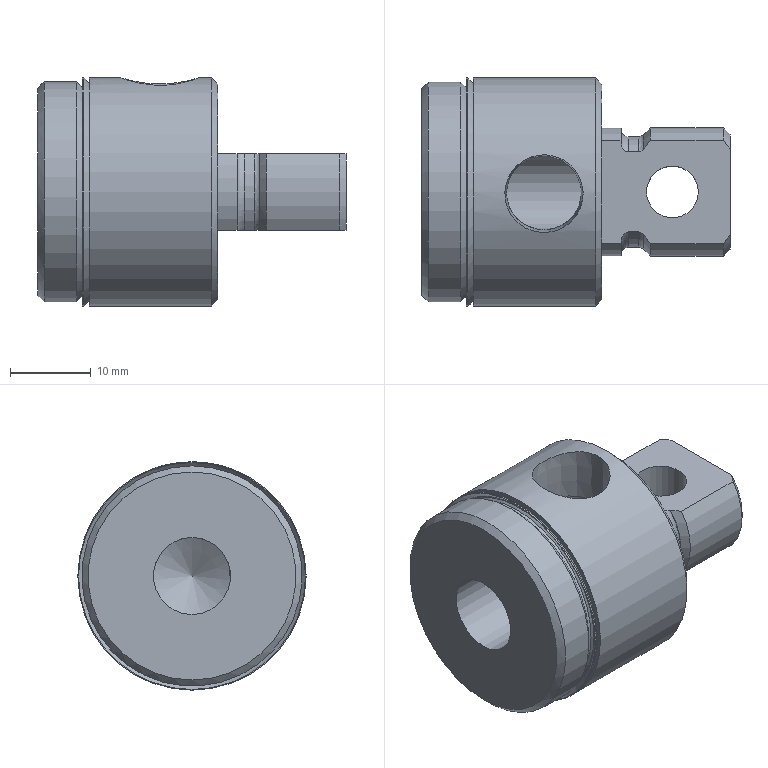Part | NX | features solid 2 | 1 solid | 41 faces | box 38.1 x 28.219 x 28.219 mm | volume 13145 mm3 | cone 14 | cylinder 13 | plane 9 | torus 5 | commonest cylinder face diameters 13.678 x2 15.812 x2 15.875 x2 28.219 x2 6.401 x1 9.246 x1
STEP:
#1=CARTESIAN_POINT('',(22.225,6.334,4.731));
#2=VERTEX_POINT('',#1);
#3=CARTESIAN_POINT('',(22.225,-6.334,4.731));
#4=VERTEX_POINT('',#3);
#5=CARTESIAN_POINT('',(22.225,28.219,4.731));
#6=DIRECTION('',(0.,-1.,0.));
#7=VECTOR('',#6,1000.);
#8=LINE('',#5,#7);
#9=EDGE_CURVE('',#2,#4,#8,.T.);
#10=ORIENTED_EDGE('',*,*,#9,.T.);
#11=CARTESIAN_POINT('',(24.613,-6.334,4.731));
#12=VERTEX_POINT('',#11);
#13=CARTESIAN_POINT('',(38.1,-6.334,4.731));
#14=DIRECTION('',(-1.,0.,0.));
#15=VECTOR('',#14,1000.);
#16=LINE('',#13,#15);
#17=EDGE_CURVE('',#12,#4,#16,.T.);
#18=ORIENTED_EDGE('',*,*,#17,.F.);
#19=CARTESIAN_POINT('',(24.613,-6.111,4.731));
#20=VERTEX_POINT('',#19);
#21=CARTESIAN_POINT('',(24.613,7.906,4.731));
#22=DIRECTION('',(0.,-1.,0.));
#23=VECTOR('',#22,1000.);
#24=LINE('',#21,#23);
#25=EDGE_CURVE('',#20,#12,#24,.T.);
#26=ORIENTED_EDGE('',*,*,#25,.F.);
#27=CARTESIAN_POINT('',(25.502,-4.939,4.731));
#28=VERTEX_POINT('',#27);
#29=CARTESIAN_POINT('',(24.613,-6.111,4.731));
#30=CARTESIAN_POINT('',(24.613,-5.842,4.731));
#31=CARTESIAN_POINT('',(24.751,-5.3,4.731));
#32=CARTESIAN_POINT('',(25.231,-4.939,4.731));
#33=CARTESIAN_POINT('',(25.502,-4.939,4.731));
#34=B_SPLINE_CURVE_WITH_KNOTS('',3,(#29,#30,#31,#32,#33),.UNSPECIFIED.,.F.,.F.,(4,1,4),(0.001401,0.002207,0.003014),.UNSPECIFIED.);
#35=EDGE_CURVE('',#20,#28,#34,.T.);
#36=ORIENTED_EDGE('',*,*,#35,.T.);
#37=CARTESIAN_POINT('',(26.784,-4.939,4.731));
#38=VERTEX_POINT('',#37);
#39=CARTESIAN_POINT('',(38.1,-4.939,4.731));
#40=DIRECTION('',(-1.,0.,0.));
#41=VECTOR('',#40,1000.);
#42=LINE('',#39,#41);
#43=EDGE_CURVE('',#38,#28,#42,.T.);
#44=ORIENTED_EDGE('',*,*,#43,.F.);
#45=CARTESIAN_POINT('',(27.383,-5.255,4.731));
#46=VERTEX_POINT('',#45);
#47=CARTESIAN_POINT('',(26.784,-4.939,4.731));
#48=CARTESIAN_POINT('',(27.017,-4.939,4.731));
#49=CARTESIAN_POINT('',(27.235,-5.073,4.731));
#50=CARTESIAN_POINT('',(27.383,-5.255,4.731));
#51=B_SPLINE_CURVE_WITH_KNOTS('',3,(#47,#48,#49,#50),.UNSPECIFIED.,.F.,.F.,(4,4),(0.003812,0.004508),.UNSPECIFIED.);
#52=EDGE_CURVE('',#38,#46,#51,.T.);
#53=ORIENTED_EDGE('',*,*,#52,.T.);
#54=CARTESIAN_POINT('',(27.413,-5.292,4.731));
#55=VERTEX_POINT('',#54);
#56=CARTESIAN_POINT('',(27.413,-5.292,4.731));
#57=CARTESIAN_POINT('',(27.403,-5.279,4.731));
#58=CARTESIAN_POINT('',(27.393,-5.267,4.731));
#59=CARTESIAN_POINT('',(27.383,-5.255,4.731));
#60=B_SPLINE_CURVE_WITH_KNOTS('',3,(#56,#57,#58,#59),.UNSPECIFIED.,.F.,.F.,(4,4),(0.01225,0.0123),.UNSPECIFIED.);
#61=EDGE_CURVE('',#55,#46,#60,.T.);
#62=ORIENTED_EDGE('',*,*,#61,.F.);
#63=CARTESIAN_POINT('',(28.252,-6.374,4.731));
#64=VERTEX_POINT('',#63);
#65=CARTESIAN_POINT('',(28.252,-6.374,4.731));
#66=CARTESIAN_POINT('',(27.967,-6.018,4.731));
#67=CARTESIAN_POINT('',(27.686,-5.658,4.731));
#68=CARTESIAN_POINT('',(27.413,-5.292,4.731));
#69=B_SPLINE_CURVE_WITH_KNOTS('',3,(#65,#66,#67,#68),.UNSPECIFIED.,.F.,.F.,(4,4),(0.01415,0.01552),.UNSPECIFIED.);
#70=EDGE_CURVE('',#64,#55,#69,.T.);
#71=ORIENTED_EDGE('',*,*,#70,.F.);
#72=CARTESIAN_POINT('',(37.261,-6.374,4.731));
#73=VERTEX_POINT('',#72);
#74=CARTESIAN_POINT('',(38.1,-6.374,4.731));
#75=DIRECTION('',(-1.,0.,0.));
#76=VECTOR('',#75,1000.);
#77=LINE('',#74,#76);
#78=EDGE_CURVE('',#73,#64,#77,.T.);
#79=ORIENTED_EDGE('',*,*,#78,.F.);
#80=CARTESIAN_POINT('',(38.1,-5.292,4.731));
#81=VERTEX_POINT('',#80);
#82=CARTESIAN_POINT('',(38.1,-5.292,4.731));
#83=CARTESIAN_POINT('',(37.828,-5.657,4.731));
#84=CARTESIAN_POINT('',(37.547,-6.017,4.731));
#85=CARTESIAN_POINT('',(37.261,-6.374,4.731));
#86=B_SPLINE_CURVE_WITH_KNOTS('',3,(#82,#83,#84,#85),.UNSPECIFIED.,.F.,.F.,(4,4),(0.02732,0.02869),.UNSPECIFIED.);
#87=EDGE_CURVE('',#81,#73,#86,.T.);
#88=ORIENTED_EDGE('',*,*,#87,.F.);
#89=CARTESIAN_POINT('',(38.1,5.292,4.731));
#90=VERTEX_POINT('',#89);
#91=CARTESIAN_POINT('',(38.1,28.219,4.731));
#92=DIRECTION('',(0.,-1.,0.));
#93=VECTOR('',#92,1000.);
#94=LINE('',#91,#93);
#95=EDGE_CURVE('',#90,#81,#94,.T.);
#96=ORIENTED_EDGE('',*,*,#95,.F.);
#97=CARTESIAN_POINT('',(37.261,6.374,4.731));
#98=VERTEX_POINT('',#97);
#99=CARTESIAN_POINT('',(37.261,6.374,4.731));
#100=CARTESIAN_POINT('',(37.546,6.018,4.731));
#101=CARTESIAN_POINT('',(37.827,5.658,4.731));
#102=CARTESIAN_POINT('',(38.1,5.292,4.731));
#103=B_SPLINE_CURVE_WITH_KNOTS('',3,(#99,#100,#101,#102),.UNSPECIFIED.,.F.,.F.,(4,4),(0.01415,0.01552),.UNSPECIFIED.);
#104=EDGE_CURVE('',#98,#90,#103,.T.);
#105=ORIENTED_EDGE('',*,*,#104,.F.);
#106=CARTESIAN_POINT('',(28.252,6.374,4.731));
#107=VERTEX_POINT('',#106);
#108=CARTESIAN_POINT('',(38.1,6.374,4.731));
#109=DIRECTION('',(-1.,0.,0.));
#110=VECTOR('',#109,1000.);
#111=LINE('',#108,#110);
#112=EDGE_CURVE('',#107,#98,#111,.F.);
#113=ORIENTED_EDGE('',*,*,#112,.F.);
#114=CARTESIAN_POINT('',(27.413,5.292,4.731));
#115=VERTEX_POINT('',#114);
#116=CARTESIAN_POINT('',(27.413,5.292,4.731));
#117=CARTESIAN_POINT('',(27.685,5.657,4.731));
#118=CARTESIAN_POINT('',(27.966,6.017,4.731));
#119=CARTESIAN_POINT('',(28.252,6.374,4.731));
#120=B_SPLINE_CURVE_WITH_KNOTS('',3,(#116,#117,#118,#119),.UNSPECIFIED.,.F.,.F.,(4,4),(0.02732,0.02869),.UNSPECIFIED.);
#121=EDGE_CURVE('',#115,#107,#120,.T.);
#122=ORIENTED_EDGE('',*,*,#121,.F.);
#123=CARTESIAN_POINT('',(27.383,5.255,4.731));
#124=VERTEX_POINT('',#123);
#125=CARTESIAN_POINT('',(27.383,5.255,4.731));
#126=CARTESIAN_POINT('',(27.393,5.267,4.731));
#127=CARTESIAN_POINT('',(27.403,5.279,4.731));
#128=CARTESIAN_POINT('',(27.413,5.292,4.731));
#129=B_SPLINE_CURVE_WITH_KNOTS('',3,(#125,#126,#127,#128),.UNSPECIFIED.,.F.,.F.,(4,4),(0.02417,0.02422),.UNSPECIFIED.);
#130=EDGE_CURVE('',#124,#115,#129,.T.);
#131=ORIENTED_EDGE('',*,*,#130,.F.);
#132=CARTESIAN_POINT('',(26.784,4.939,4.731));
#133=VERTEX_POINT('',#132);
#134=CARTESIAN_POINT('',(27.383,5.255,4.731));
#135=CARTESIAN_POINT('',(27.236,5.075,4.731));
#136=CARTESIAN_POINT('',(27.018,4.939,4.731));
#137=CARTESIAN_POINT('',(26.784,4.939,4.731));
#138=B_SPLINE_CURVE_WITH_KNOTS('',3,(#134,#135,#136,#137),.UNSPECIFIED.,.F.,.F.,(4,4),(0.005905,0.0066),.UNSPECIFIED.);
#139=EDGE_CURVE('',#124,#133,#138,.T.);
#140=ORIENTED_EDGE('',*,*,#139,.T.);
#141=CARTESIAN_POINT('',(25.502,4.939,4.731));
#142=VERTEX_POINT('',#141);
#143=CARTESIAN_POINT('',(38.1,4.939,4.731));
#144=DIRECTION('',(-1.,0.,0.));
#145=VECTOR('',#144,1000.);
#146=LINE('',#143,#145);
#147=EDGE_CURVE('',#142,#133,#146,.F.);
#148=ORIENTED_EDGE('',*,*,#147,.F.);
#149=CARTESIAN_POINT('',(24.613,6.111,4.731));
#150=VERTEX_POINT('',#149);
#151=CARTESIAN_POINT('',(25.502,4.939,4.731));
#152=CARTESIAN_POINT('',(25.232,4.939,4.731));
#153=CARTESIAN_POINT('',(24.751,5.299,4.731));
#154=CARTESIAN_POINT('',(24.613,5.842,4.731));
#155=CARTESIAN_POINT('',(24.613,6.111,4.731));
#156=B_SPLINE_CURVE_WITH_KNOTS('',3,(#151,#152,#153,#154,#155),.UNSPECIFIED.,.F.,.F.,(4,1,4),(0.006205,0.007011,0.007818),.UNSPECIFIED.);
#157=EDGE_CURVE('',#142,#150,#156,.T.);
#158=ORIENTED_EDGE('',*,*,#157,.T.);
#159=CARTESIAN_POINT('',(24.613,6.334,4.731));
#160=VERTEX_POINT('',#159);
#161=CARTESIAN_POINT('',(24.613,7.906,4.731));
#162=DIRECTION('',(0.,-1.,0.));
#163=VECTOR('',#162,1000.);
#164=LINE('',#161,#163);
#165=EDGE_CURVE('',#160,#150,#164,.T.);
#166=ORIENTED_EDGE('',*,*,#165,.F.);
#167=CARTESIAN_POINT('',(38.1,6.334,4.731));
#168=DIRECTION('',(-1.,0.,0.));
#169=VECTOR('',#168,1000.);
#170=LINE('',#167,#169);
#171=EDGE_CURVE('',#2,#160,#170,.F.);
#172=ORIENTED_EDGE('',*,*,#171,.F.);
#173=EDGE_LOOP('',(#10,#18,#26,#36,#44,#53,#62,#71,#79,#88,#96,#105,#113,#122,#131,#140,#148,#158,#166,#172));
#174=FACE_BOUND('',#173,.T.);
#175=CARTESIAN_POINT('',(34.163,0.,4.731));
#176=VERTEX_POINT('',#175);
#177=CARTESIAN_POINT('',(30.963,0.,4.731));
#178=DIRECTION('',(0.,0.,1.));
#179=DIRECTION('',(1.,0.,0.));
#180=AXIS2_PLACEMENT_3D('',#177,#178,#179);
#181=CIRCLE('',#180,3.2);
#182=EDGE_CURVE('',#176,#176,#181,.F.);
#183=ORIENTED_EDGE('',*,*,#182,.T.);
#184=EDGE_LOOP('',(#183));
#185=FACE_BOUND('',#184,.T.);
#186=CARTESIAN_POINT('',(22.225,28.219,4.731));
#187=DIRECTION('',(0.,0.,1.));
#188=DIRECTION('',(1.,0.,0.));
#189=AXIS2_PLACEMENT_3D('',#186,#187,#188);
#190=PLANE('',#189);
#191=ADVANCED_FACE('',(#174,#185),#190,.T.);
#192=CARTESIAN_POINT('',(22.225,-6.334,-4.731));
#193=VERTEX_POINT('',#192);
#194=CARTESIAN_POINT('',(22.225,6.334,-4.731));
#195=VERTEX_POINT('',#194);
#196=CARTESIAN_POINT('',(22.225,-28.219,-4.731));
#197=DIRECTION('',(0.,1.,0.));
#198=VECTOR('',#197,1000.);
#199=LINE('',#196,#198);
#200=EDGE_CURVE('',#193,#195,#199,.T.);
#201=ORIENTED_EDGE('',*,*,#200,.T.);
#202=CARTESIAN_POINT('',(24.613,6.334,-4.731));
#203=VERTEX_POINT('',#202);
#204=CARTESIAN_POINT('',(38.1,6.334,-4.731));
#205=DIRECTION('',(-1.,0.,0.));
#206=VECTOR('',#205,1000.);
#207=LINE('',#204,#206);
#208=EDGE_CURVE('',#203,#195,#207,.T.);
#209=ORIENTED_EDGE('',*,*,#208,.F.);
#210=CARTESIAN_POINT('',(24.613,6.111,-4.731));
#211=VERTEX_POINT('',#210);
#212=CARTESIAN_POINT('',(24.613,7.906,-4.731));
#213=DIRECTION('',(0.,1.,0.));
#214=VECTOR('',#213,1000.);
#215=LINE('',#212,#214);
#216=EDGE_CURVE('',#211,#203,#215,.T.);
#217=ORIENTED_EDGE('',*,*,#216,.F.);
#218=CARTESIAN_POINT('',(25.502,4.939,-4.731));
#219=VERTEX_POINT('',#218);
#220=CARTESIAN_POINT('',(24.613,6.111,-4.731));
#221=CARTESIAN_POINT('',(24.613,5.839,-4.731));
#222=CARTESIAN_POINT('',(24.75,5.302,-4.731));
#223=CARTESIAN_POINT('',(25.232,4.939,-4.731));
#224=CARTESIAN_POINT('',(25.502,4.939,-4.731));
#225=B_SPLINE_CURVE_WITH_KNOTS('',3,(#220,#221,#222,#223,#224),.UNSPECIFIED.,.F.,.F.,(4,1,4),(0.004854,0.005662,0.006469),.UNSPECIFIED.);
#226=EDGE_CURVE('',#211,#219,#225,.T.);
#227=ORIENTED_EDGE('',*,*,#226,.T.);
#228=CARTESIAN_POINT('',(26.784,4.939,-4.731));
#229=VERTEX_POINT('',#228);
#230=CARTESIAN_POINT('',(38.1,4.939,-4.731));
#231=DIRECTION('',(-1.,0.,0.));
#232=VECTOR('',#231,1000.);
#233=LINE('',#230,#232);
#234=EDGE_CURVE('',#229,#219,#233,.T.);
#235=ORIENTED_EDGE('',*,*,#234,.F.);
#236=CARTESIAN_POINT('',(27.383,5.255,-4.731));
#237=VERTEX_POINT('',#236);
#238=CARTESIAN_POINT('',(26.784,4.939,-4.731));
#239=CARTESIAN_POINT('',(27.017,4.939,-4.731));
#240=CARTESIAN_POINT('',(27.237,5.076,-4.731));
#241=CARTESIAN_POINT('',(27.383,5.255,-4.731));
#242=B_SPLINE_CURVE_WITH_KNOTS('',3,(#238,#239,#240,#241),.UNSPECIFIED.,.F.,.F.,(4,4),(0.00608,0.006774),.UNSPECIFIED.);
#243=EDGE_CURVE('',#229,#237,#242,.T.);
#244=ORIENTED_EDGE('',*,*,#243,.T.);
#245=CARTESIAN_POINT('',(27.413,5.292,-4.731));
#246=VERTEX_POINT('',#245);
#247=CARTESIAN_POINT('',(27.413,5.292,-4.731));
#248=CARTESIAN_POINT('',(27.403,5.279,-4.731));
#249=CARTESIAN_POINT('',(27.393,5.267,-4.731));
#250=CARTESIAN_POINT('',(27.383,5.255,-4.731));
#251=B_SPLINE_CURVE_WITH_KNOTS('',3,(#247,#248,#249,#250),.UNSPECIFIED.,.F.,.F.,(4,4),(0.01225,0.0123),.UNSPECIFIED.);
#252=EDGE_CURVE('',#246,#237,#251,.T.);
#253=ORIENTED_EDGE('',*,*,#252,.F.);
#254=CARTESIAN_POINT('',(28.252,6.374,-4.731));
#255=VERTEX_POINT('',#254);
#256=CARTESIAN_POINT('',(28.252,6.374,-4.731));
#257=CARTESIAN_POINT('',(27.967,6.018,-4.731));
#258=CARTESIAN_POINT('',(27.686,5.658,-4.731));
#259=CARTESIAN_POINT('',(27.413,5.292,-4.731));
#260=B_SPLINE_CURVE_WITH_KNOTS('',3,(#256,#257,#258,#259),.UNSPECIFIED.,.F.,.F.,(4,4),(0.01415,0.01552),.UNSPECIFIED.);
#261=EDGE_CURVE('',#255,#246,#260,.T.);
#262=ORIENTED_EDGE('',*,*,#261,.F.);
#263=CARTESIAN_POINT('',(37.261,6.374,-4.731));
#264=VERTEX_POINT('',#263);
#265=CARTESIAN_POINT('',(38.1,6.374,-4.731));
#266=DIRECTION('',(-1.,0.,0.));
#267=VECTOR('',#266,1000.);
#268=LINE('',#265,#267);
#269=EDGE_CURVE('',#264,#255,#268,.T.);
#270=ORIENTED_EDGE('',*,*,#269,.F.);
#271=CARTESIAN_POINT('',(38.1,5.292,-4.731));
#272=VERTEX_POINT('',#271);
#273=CARTESIAN_POINT('',(38.1,5.292,-4.731));
#274=CARTESIAN_POINT('',(37.828,5.657,-4.731));
#275=CARTESIAN_POINT('',(37.547,6.017,-4.731));
#276=CARTESIAN_POINT('',(37.261,6.374,-4.731));
#277=B_SPLINE_CURVE_WITH_KNOTS('',3,(#273,#274,#275,#276),.UNSPECIFIED.,.F.,.F.,(4,4),(0.02732,0.02869),.UNSPECIFIED.);
#278=EDGE_CURVE('',#272,#264,#277,.T.);
#279=ORIENTED_EDGE('',*,*,#278,.F.);
#280=CARTESIAN_POINT('',(38.1,-5.292,-4.731));
#281=VERTEX_POINT('',#280);
#282=CARTESIAN_POINT('',(38.1,-28.219,-4.731));
#283=DIRECTION('',(0.,1.,0.));
#284=VECTOR('',#283,1000.);
#285=LINE('',#282,#284);
#286=EDGE_CURVE('',#281,#272,#285,.T.);
#287=ORIENTED_EDGE('',*,*,#286,.F.);
#288=CARTESIAN_POINT('',(37.261,-6.374,-4.731));
#289=VERTEX_POINT('',#288);
#290=CARTESIAN_POINT('',(37.261,-6.374,-4.731));
#291=CARTESIAN_POINT('',(37.546,-6.018,-4.731));
#292=CARTESIAN_POINT('',(37.827,-5.658,-4.731));
#293=CARTESIAN_POINT('',(38.1,-5.292,-4.731));
#294=B_SPLINE_CURVE_WITH_KNOTS('',3,(#290,#291,#292,#293),.UNSPECIFIED.,.F.,.F.,(4,4),(0.01415,0.01552),.UNSPECIFIED.);
#295=EDGE_CURVE('',#289,#281,#294,.T.);
#296=ORIENTED_EDGE('',*,*,#295,.F.);
#297=CARTESIAN_POINT('',(28.252,-6.374,-4.731));
#298=VERTEX_POINT('',#297);
#299=CARTESIAN_POINT('',(38.1,-6.374,-4.731));
#300=DIRECTION('',(-1.,0.,0.));
#301=VECTOR('',#300,1000.);
#302=LINE('',#299,#301);
#303=EDGE_CURVE('',#298,#289,#302,.F.);
#304=ORIENTED_EDGE('',*,*,#303,.F.);
#305=CARTESIAN_POINT('',(27.413,-5.292,-4.731));
#306=VERTEX_POINT('',#305);
#307=CARTESIAN_POINT('',(27.413,-5.292,-4.731));
#308=CARTESIAN_POINT('',(27.685,-5.657,-4.731));
#309=CARTESIAN_POINT('',(27.966,-6.017,-4.731));
#310=CARTESIAN_POINT('',(28.252,-6.374,-4.731));
#311=B_SPLINE_CURVE_WITH_KNOTS('',3,(#307,#308,#309,#310),.UNSPECIFIED.,.F.,.F.,(4,4),(0.02732,0.02869),.UNSPECIFIED.);
#312=EDGE_CURVE('',#306,#298,#311,.T.);
#313=ORIENTED_EDGE('',*,*,#312,.F.);
#314=CARTESIAN_POINT('',(27.383,-5.255,-4.731));
#315=VERTEX_POINT('',#314);
#316=CARTESIAN_POINT('',(27.383,-5.255,-4.731));
#317=CARTESIAN_POINT('',(27.393,-5.267,-4.731));
#318=CARTESIAN_POINT('',(27.403,-5.279,-4.731));
#319=CARTESIAN_POINT('',(27.413,-5.292,-4.731));
#320=B_SPLINE_CURVE_WITH_KNOTS('',3,(#316,#317,#318,#319),.UNSPECIFIED.,.F.,.F.,(4,4),(0.02417,0.02422),.UNSPECIFIED.);
#321=EDGE_CURVE('',#315,#306,#320,.T.);
#322=ORIENTED_EDGE('',*,*,#321,.F.);
#323=CARTESIAN_POINT('',(26.784,-4.939,-4.731));
#324=VERTEX_POINT('',#323);
#325=CARTESIAN_POINT('',(27.383,-5.255,-4.731));
#326=CARTESIAN_POINT('',(27.236,-5.075,-4.731));
#327=CARTESIAN_POINT('',(27.017,-4.939,-4.731));
#328=CARTESIAN_POINT('',(26.784,-4.939,-4.731));
#329=B_SPLINE_CURVE_WITH_KNOTS('',3,(#325,#326,#327,#328),.UNSPECIFIED.,.F.,.F.,(4,4),(0.00183,0.002524),.UNSPECIFIED.);
#330=EDGE_CURVE('',#315,#324,#329,.T.);
#331=ORIENTED_EDGE('',*,*,#330,.T.);
#332=CARTESIAN_POINT('',(25.502,-4.939,-4.731));
#333=VERTEX_POINT('',#332);
#334=CARTESIAN_POINT('',(38.1,-4.939,-4.731));
#335=DIRECTION('',(-1.,0.,0.));
#336=VECTOR('',#335,1000.);
#337=LINE('',#334,#336);
#338=EDGE_CURVE('',#333,#324,#337,.F.);
#339=ORIENTED_EDGE('',*,*,#338,.F.);
#340=CARTESIAN_POINT('',(24.613,-6.111,-4.731));
#341=VERTEX_POINT('',#340);
#342=CARTESIAN_POINT('',(25.502,-4.939,-4.731));
#343=CARTESIAN_POINT('',(25.233,-4.939,-4.731));
#344=CARTESIAN_POINT('',(24.751,-5.299,-4.731));
#345=CARTESIAN_POINT('',(24.613,-5.843,-4.731));
#346=CARTESIAN_POINT('',(24.613,-6.111,-4.731));
#347=B_SPLINE_CURVE_WITH_KNOTS('',3,(#342,#343,#344,#345,#346),.UNSPECIFIED.,.F.,.F.,(4,1,4),(0.003324,0.004131,0.004938),.UNSPECIFIED.);
#348=EDGE_CURVE('',#333,#341,#347,.T.);
#349=ORIENTED_EDGE('',*,*,#348,.T.);
#350=CARTESIAN_POINT('',(24.613,-6.334,-4.731));
#351=VERTEX_POINT('',#350);
#352=CARTESIAN_POINT('',(24.613,7.906,-4.731));
#353=DIRECTION('',(0.,1.,0.));
#354=VECTOR('',#353,1000.);
#355=LINE('',#352,#354);
#356=EDGE_CURVE('',#351,#341,#355,.T.);
#357=ORIENTED_EDGE('',*,*,#356,.F.);
#358=CARTESIAN_POINT('',(38.1,-6.334,-4.731));
#359=DIRECTION('',(-1.,0.,0.));
#360=VECTOR('',#359,1000.);
#361=LINE('',#358,#360);
#362=EDGE_CURVE('',#193,#351,#361,.F.);
#363=ORIENTED_EDGE('',*,*,#362,.F.);
#364=EDGE_LOOP('',(#201,#209,#217,#227,#235,#244,#253,#262,#270,#279,#287,#296,#304,#313,#322,#331,#339,#349,#357,#363));
#365=FACE_BOUND('',#364,.T.);
#366=CARTESIAN_POINT('',(27.762,0.,-4.731));
#367=VERTEX_POINT('',#366);
#368=CARTESIAN_POINT('',(30.963,0.,-4.731));
#369=DIRECTION('',(0.,0.,-1.));
#370=DIRECTION('',(-1.,0.,0.));
#371=AXIS2_PLACEMENT_3D('',#368,#369,#370);
#372=CIRCLE('',#371,3.2);
#373=EDGE_CURVE('',#367,#367,#372,.F.);
#374=ORIENTED_EDGE('',*,*,#373,.T.);
#375=EDGE_LOOP('',(#374));
#376=FACE_BOUND('',#375,.T.);
#377=CARTESIAN_POINT('',(22.225,-28.219,-4.731));
#378=DIRECTION('',(0.,0.,-1.));
#379=DIRECTION('',(-1.,0.,0.));
#380=AXIS2_PLACEMENT_3D('',#377,#378,#379);
#381=PLANE('',#380);
#382=ADVANCED_FACE('',(#365,#376),#381,.T.);
#383=CARTESIAN_POINT('',(5.588,0.,12.846));
#384=VERTEX_POINT('',#383);
#385=CARTESIAN_POINT('',(5.588,0.,0.));
#386=DIRECTION('',(-1.,0.,0.));
#387=DIRECTION('',(0.,0.,1.));
#388=AXIS2_PLACEMENT_3D('',#385,#386,#387);
#389=CIRCLE('',#388,12.846);
#390=EDGE_CURVE('',#384,#384,#389,.T.);
#391=ORIENTED_EDGE('',*,*,#390,.F.);
#392=EDGE_LOOP('',(#391));
#393=FACE_BOUND('',#392,.T.);
#394=CARTESIAN_POINT('',(5.969,-12.846,0.));
#395=VERTEX_POINT('',#394);
#396=CARTESIAN_POINT('',(5.969,0.,0.));
#397=DIRECTION('',(-1.,0.,0.));
#398=DIRECTION('',(0.,-1.,0.));
#399=AXIS2_PLACEMENT_3D('',#396,#397,#398);
#400=CIRCLE('',#399,12.846);
#401=EDGE_CURVE('',#395,#395,#400,.T.);
#402=ORIENTED_EDGE('',*,*,#401,.T.);
#403=EDGE_LOOP('',(#402));
#404=FACE_BOUND('',#403,.T.);
#405=CARTESIAN_POINT('',(22.225,0.,0.));
#406=DIRECTION('',(-1.,0.,0.));
#407=DIRECTION('',(0.,0.,1.));
#408=AXIS2_PLACEMENT_3D('',#405,#406,#407);
#409=CYLINDRICAL_SURFACE('',#408,12.846);
#410=ADVANCED_FACE('',(#393,#404),#409,.T.);
#411=CARTESIAN_POINT('',(6.35,0.,14.11));
#412=VERTEX_POINT('',#411);
#413=CARTESIAN_POINT('',(6.35,0.,0.));
#414=DIRECTION('',(-1.,0.,0.));
#415=DIRECTION('',(0.,0.,1.));
#416=AXIS2_PLACEMENT_3D('',#413,#414,#415);
#417=CIRCLE('',#416,14.11);
#418=EDGE_CURVE('',#412,#412,#417,.T.);
#419=ORIENTED_EDGE('',*,*,#418,.T.);
#420=EDGE_LOOP('',(#419));
#421=FACE_BOUND('',#420,.T.);
#422=CARTESIAN_POINT('',(6.35,-13.449,0.));
#423=VERTEX_POINT('',#422);
#424=CARTESIAN_POINT('',(6.35,0.,0.));
#425=DIRECTION('',(-1.,0.,0.));
#426=DIRECTION('',(0.,-1.,0.));
#427=AXIS2_PLACEMENT_3D('',#424,#425,#426);
#428=CIRCLE('',#427,13.449);
#429=EDGE_CURVE('',#423,#423,#428,.T.);
#430=ORIENTED_EDGE('',*,*,#429,.F.);
#431=EDGE_LOOP('',(#430));
#432=FACE_BOUND('',#431,.T.);
#433=CARTESIAN_POINT('',(6.35,12.846,0.));
#434=DIRECTION('',(-1.,0.,0.));
#435=DIRECTION('',(0.,0.,1.));
#436=AXIS2_PLACEMENT_3D('',#433,#434,#435);
#437=PLANE('',#436);
#438=ADVANCED_FACE('',(#421,#432),#437,.T.);
#439=CARTESIAN_POINT('',(22.225,0.,0.));
#440=DIRECTION('',(1.,0.,0.));
#441=DIRECTION('',(0.,0.,-1.));
#442=AXIS2_PLACEMENT_3D('',#439,#440,#441);
#443=CIRCLE('',#442,7.906);
#444=EDGE_CURVE('',#4,#193,#443,.T.);
#445=ORIENTED_EDGE('',*,*,#444,.T.);
#446=ORIENTED_EDGE('',*,*,#362,.T.);
#447=CARTESIAN_POINT('',(24.613,0.,0.));
#448=DIRECTION('',(-1.,0.,0.));
#449=DIRECTION('',(0.,0.,1.));
#450=AXIS2_PLACEMENT_3D('',#447,#448,#449);
#451=CIRCLE('',#450,7.906);
#452=EDGE_CURVE('',#351,#12,#451,.T.);
#453=ORIENTED_EDGE('',*,*,#452,.T.);
#454=ORIENTED_EDGE('',*,*,#17,.T.);
#455=EDGE_LOOP('',(#445,#446,#453,#454));
#456=FACE_BOUND('',#455,.T.);
#457=CARTESIAN_POINT('',(38.1,0.,0.));
#458=DIRECTION('',(-1.,0.,0.));
#459=DIRECTION('',(0.,0.,1.));
#460=AXIS2_PLACEMENT_3D('',#457,#458,#459);
#461=CYLINDRICAL_SURFACE('',#460,7.906);
#462=ADVANCED_FACE('',(#456),#461,.T.);
#463=CARTESIAN_POINT('',(24.613,0.,0.));
#464=DIRECTION('',(-1.,0.,0.));
#465=DIRECTION('',(0.,0.,1.));
#466=AXIS2_PLACEMENT_3D('',#463,#464,#465);
#467=CIRCLE('',#466,7.906);
#468=EDGE_CURVE('',#160,#203,#467,.T.);
#469=ORIENTED_EDGE('',*,*,#468,.T.);
#470=ORIENTED_EDGE('',*,*,#208,.T.);
#471=CARTESIAN_POINT('',(22.225,0.,0.));
#472=DIRECTION('',(1.,0.,0.));
#473=DIRECTION('',(0.,0.,-1.));
#474=AXIS2_PLACEMENT_3D('',#471,#472,#473);
#475=CIRCLE('',#474,7.906);
#476=EDGE_CURVE('',#195,#2,#475,.T.);
#477=ORIENTED_EDGE('',*,*,#476,.T.);
#478=ORIENTED_EDGE('',*,*,#171,.T.);
#479=EDGE_LOOP('',(#469,#470,#477,#478));
#480=FACE_BOUND('',#479,.T.);
#481=CARTESIAN_POINT('',(38.1,0.,0.));
#482=DIRECTION('',(-1.,0.,0.));
#483=DIRECTION('',(0.,0.,1.));
#484=AXIS2_PLACEMENT_3D('',#481,#482,#483);
#485=CYLINDRICAL_SURFACE('',#484,7.906);
#486=ADVANCED_FACE('',(#480),#485,.T.);
#487=ORIENTED_EDGE('',*,*,#452,.F.);
#488=ORIENTED_EDGE('',*,*,#356,.T.);
#489=CARTESIAN_POINT('',(24.613,0.,0.));
#490=DIRECTION('',(-1.,0.,0.));
#491=DIRECTION('',(0.,0.,1.));
#492=AXIS2_PLACEMENT_3D('',#489,#490,#491);
#493=CIRCLE('',#492,7.728);
#494=EDGE_CURVE('',#341,#20,#493,.T.);
#495=ORIENTED_EDGE('',*,*,#494,.T.);
#496=ORIENTED_EDGE('',*,*,#25,.T.);
#497=EDGE_LOOP('',(#487,#488,#495,#496));
#498=FACE_BOUND('',#497,.T.);
#499=CARTESIAN_POINT('',(24.613,7.906,0.));
#500=DIRECTION('',(1.,0.,0.));
#501=DIRECTION('',(0.,0.,-1.));
#502=AXIS2_PLACEMENT_3D('',#499,#500,#501);
#503=PLANE('',#502);
#504=ADVANCED_FACE('',(#498),#503,.T.);
#505=CARTESIAN_POINT('',(24.613,0.,0.));
#506=DIRECTION('',(-1.,0.,0.));
#507=DIRECTION('',(0.,0.,1.));
#508=AXIS2_PLACEMENT_3D('',#505,#506,#507);
#509=CIRCLE('',#508,7.728);
#510=EDGE_CURVE('',#150,#211,#509,.T.);
#511=ORIENTED_EDGE('',*,*,#510,.T.);
#512=ORIENTED_EDGE('',*,*,#216,.T.);
#513=ORIENTED_EDGE('',*,*,#468,.F.);
#514=ORIENTED_EDGE('',*,*,#165,.T.);
#515=EDGE_LOOP('',(#511,#512,#513,#514));
#516=FACE_BOUND('',#515,.T.);
#517=CARTESIAN_POINT('',(24.613,7.906,0.));
#518=DIRECTION('',(1.,0.,0.));
#519=DIRECTION('',(0.,0.,-1.));
#520=AXIS2_PLACEMENT_3D('',#517,#518,#519);
#521=PLANE('',#520);
#522=ADVANCED_FACE('',(#516),#521,.T.);
#523=ORIENTED_EDGE('',*,*,#348,.F.);
#524=CARTESIAN_POINT('',(25.502,0.,0.));
#525=DIRECTION('',(-1.,0.,0.));
#526=DIRECTION('',(0.,0.,1.));
#527=AXIS2_PLACEMENT_3D('',#524,#525,#526);
#528=CIRCLE('',#527,6.839);
#529=EDGE_CURVE('',#333,#28,#528,.T.);
#530=ORIENTED_EDGE('',*,*,#529,.T.);
#531=ORIENTED_EDGE('',*,*,#35,.F.);
#532=ORIENTED_EDGE('',*,*,#494,.F.);
#533=EDGE_LOOP('',(#523,#530,#531,#532));
#534=FACE_BOUND('',#533,.T.);
#535=CARTESIAN_POINT('',(25.502,0.,0.));
#536=DIRECTION('',(-1.,0.,0.));
#537=DIRECTION('',(0.,0.,1.));
#538=AXIS2_PLACEMENT_3D('',#535,#536,#537);
#539=TOROIDAL_SURFACE('',#538,7.728,0.889);
#540=ADVANCED_FACE('',(#534),#539,.F.);
#541=ORIENTED_EDGE('',*,*,#226,.F.);
#542=ORIENTED_EDGE('',*,*,#510,.F.);
#543=ORIENTED_EDGE('',*,*,#157,.F.);
#544=CARTESIAN_POINT('',(25.502,0.,0.));
#545=DIRECTION('',(-1.,0.,0.));
#546=DIRECTION('',(0.,0.,1.));
#547=AXIS2_PLACEMENT_3D('',#544,#545,#546);
#548=CIRCLE('',#547,6.839);
#549=EDGE_CURVE('',#142,#219,#548,.T.);
#550=ORIENTED_EDGE('',*,*,#549,.T.);
#551=EDGE_LOOP('',(#541,#542,#543,#550));
#552=FACE_BOUND('',#551,.T.);
#553=CARTESIAN_POINT('',(25.502,0.,0.));
#554=DIRECTION('',(-1.,0.,0.));
#555=DIRECTION('',(0.,0.,1.));
#556=AXIS2_PLACEMENT_3D('',#553,#554,#555);
#557=TOROIDAL_SURFACE('',#556,7.728,0.889);
#558=ADVANCED_FACE('',(#552),#557,.F.);
#559=ORIENTED_EDGE('',*,*,#529,.F.);
#560=ORIENTED_EDGE('',*,*,#338,.T.);
#561=CARTESIAN_POINT('',(26.784,0.,0.));
#562=DIRECTION('',(-1.,0.,0.));
#563=DIRECTION('',(0.,0.,1.));
#564=AXIS2_PLACEMENT_3D('',#561,#562,#563);
#565=CIRCLE('',#564,6.839);
#566=EDGE_CURVE('',#324,#38,#565,.T.);
#567=ORIENTED_EDGE('',*,*,#566,.T.);
#568=ORIENTED_EDGE('',*,*,#43,.T.);
#569=EDGE_LOOP('',(#559,#560,#567,#568));
#570=FACE_BOUND('',#569,.T.);
#571=CARTESIAN_POINT('',(38.1,0.,0.));
#572=DIRECTION('',(-1.,0.,0.));
#573=DIRECTION('',(0.,0.,1.));
#574=AXIS2_PLACEMENT_3D('',#571,#572,#573);
#575=CYLINDRICAL_SURFACE('',#574,6.839);
#576=ADVANCED_FACE('',(#570),#575,.T.);
#577=CARTESIAN_POINT('',(26.784,0.,0.));
#578=DIRECTION('',(-1.,0.,0.));
#579=DIRECTION('',(0.,0.,1.));
#580=AXIS2_PLACEMENT_3D('',#577,#578,#579);
#581=CIRCLE('',#580,6.839);
#582=EDGE_CURVE('',#133,#229,#581,.T.);
#583=ORIENTED_EDGE('',*,*,#582,.T.);
#584=ORIENTED_EDGE('',*,*,#234,.T.);
#585=ORIENTED_EDGE('',*,*,#549,.F.);
#586=ORIENTED_EDGE('',*,*,#147,.T.);
#587=EDGE_LOOP('',(#583,#584,#585,#586));
#588=FACE_BOUND('',#587,.T.);
#589=CARTESIAN_POINT('',(38.1,0.,0.));
#590=DIRECTION('',(-1.,0.,0.));
#591=DIRECTION('',(0.,0.,1.));
#592=AXIS2_PLACEMENT_3D('',#589,#590,#591);
#593=CYLINDRICAL_SURFACE('',#592,6.839);
#594=ADVANCED_FACE('',(#588),#593,.T.);
#595=ORIENTED_EDGE('',*,*,#330,.F.);
#596=CARTESIAN_POINT('',(27.383,0.,0.));
#597=DIRECTION('',(-1.,0.,0.));
#598=DIRECTION('',(0.,0.,1.));
#599=AXIS2_PLACEMENT_3D('',#596,#597,#598);
#600=CIRCLE('',#599,7.071);
#601=EDGE_CURVE('',#315,#46,#600,.T.);
#602=ORIENTED_EDGE('',*,*,#601,.T.);
#603=ORIENTED_EDGE('',*,*,#52,.F.);
#604=ORIENTED_EDGE('',*,*,#566,.F.);
#605=EDGE_LOOP('',(#595,#602,#603,#604));
#606=FACE_BOUND('',#605,.T.);
#607=CARTESIAN_POINT('',(26.784,0.,0.));
#608=DIRECTION('',(-1.,0.,0.));
#609=DIRECTION('',(0.,0.,1.));
#610=AXIS2_PLACEMENT_3D('',#607,#608,#609);
#611=TOROIDAL_SURFACE('',#610,7.728,0.889);
#612=ADVANCED_FACE('',(#606),#611,.F.);
#613=ORIENTED_EDGE('',*,*,#243,.F.);
#614=ORIENTED_EDGE('',*,*,#582,.F.);
#615=ORIENTED_EDGE('',*,*,#139,.F.);
#616=CARTESIAN_POINT('',(27.383,0.,0.));
#617=DIRECTION('',(-1.,0.,0.));
#618=DIRECTION('',(0.,0.,1.));
#619=AXIS2_PLACEMENT_3D('',#616,#617,#618);
#620=CIRCLE('',#619,7.071);
#621=EDGE_CURVE('',#124,#237,#620,.T.);
#622=ORIENTED_EDGE('',*,*,#621,.T.);
#623=EDGE_LOOP('',(#613,#614,#615,#622));
#624=FACE_BOUND('',#623,.T.);
#625=CARTESIAN_POINT('',(26.784,0.,0.));
#626=DIRECTION('',(-1.,0.,0.));
#627=DIRECTION('',(0.,0.,1.));
#628=AXIS2_PLACEMENT_3D('',#625,#626,#627);
#629=TOROIDAL_SURFACE('',#628,7.728,0.889);
#630=ADVANCED_FACE('',(#624),#629,.F.);
#631=CARTESIAN_POINT('',(27.413,0.,0.));
#632=DIRECTION('',(-1.,0.,0.));
#633=DIRECTION('',(0.,0.,1.));
#634=AXIS2_PLACEMENT_3D('',#631,#632,#633);
#635=CIRCLE('',#634,7.098);
#636=EDGE_CURVE('',#115,#246,#635,.T.);
#637=ORIENTED_EDGE('',*,*,#636,.T.);
#638=ORIENTED_EDGE('',*,*,#252,.T.);
#639=ORIENTED_EDGE('',*,*,#621,.F.);
#640=ORIENTED_EDGE('',*,*,#130,.T.);
#641=EDGE_LOOP('',(#637,#638,#639,#640));
#642=FACE_BOUND('',#641,.T.);
#643=CARTESIAN_POINT('',(27.383,0.,0.));
#644=DIRECTION('',(1.,0.,0.));
#645=DIRECTION('',(0.,0.,-1.));
#646=AXIS2_PLACEMENT_3D('',#643,#644,#645);
#647=CONICAL_SURFACE('',#646,7.071,0.7389);
#648=ADVANCED_FACE('',(#642),#647,.T.);
#649=ORIENTED_EDGE('',*,*,#601,.F.);
#650=ORIENTED_EDGE('',*,*,#321,.T.);
#651=CARTESIAN_POINT('',(27.413,0.,0.));
#652=DIRECTION('',(-1.,0.,0.));
#653=DIRECTION('',(0.,0.,1.));
#654=AXIS2_PLACEMENT_3D('',#651,#652,#653);
#655=CIRCLE('',#654,7.098);
#656=EDGE_CURVE('',#306,#55,#655,.T.);
#657=ORIENTED_EDGE('',*,*,#656,.T.);
#658=ORIENTED_EDGE('',*,*,#61,.T.);
#659=EDGE_LOOP('',(#649,#650,#657,#658));
#660=FACE_BOUND('',#659,.T.);
#661=CARTESIAN_POINT('',(27.383,0.,0.));
#662=DIRECTION('',(1.,0.,0.));
#663=DIRECTION('',(0.,0.,-1.));
#664=AXIS2_PLACEMENT_3D('',#661,#662,#663);
#665=CONICAL_SURFACE('',#664,7.071,0.7389);
#666=ADVANCED_FACE('',(#660),#665,.T.);
#667=CARTESIAN_POINT('',(28.252,0.,0.));
#668=DIRECTION('',(-1.,0.,0.));
#669=DIRECTION('',(0.,0.,1.));
#670=AXIS2_PLACEMENT_3D('',#667,#668,#669);
#671=CIRCLE('',#670,7.938);
#672=EDGE_CURVE('',#107,#255,#671,.T.);
#673=ORIENTED_EDGE('',*,*,#672,.T.);
#674=ORIENTED_EDGE('',*,*,#261,.T.);
#675=ORIENTED_EDGE('',*,*,#636,.F.);
#676=ORIENTED_EDGE('',*,*,#121,.T.);
#677=EDGE_LOOP('',(#673,#674,#675,#676));
#678=FACE_BOUND('',#677,.T.);
#679=CARTESIAN_POINT('',(27.413,0.,0.));
#680=DIRECTION('',(1.,0.,0.));
#681=DIRECTION('',(0.,0.,-1.));
#682=AXIS2_PLACEMENT_3D('',#679,#680,#681);
#683=CONICAL_SURFACE('',#682,7.098,0.7854);
#684=ADVANCED_FACE('',(#678),#683,.T.);
#685=ORIENTED_EDGE('',*,*,#656,.F.);
#686=ORIENTED_EDGE('',*,*,#312,.T.);
#687=CARTESIAN_POINT('',(28.252,0.,0.));
#688=DIRECTION('',(-1.,0.,0.));
#689=DIRECTION('',(0.,0.,1.));
#690=AXIS2_PLACEMENT_3D('',#687,#688,#689);
#691=CIRCLE('',#690,7.938);
#692=EDGE_CURVE('',#298,#64,#691,.T.);
#693=ORIENTED_EDGE('',*,*,#692,.T.);
#694=ORIENTED_EDGE('',*,*,#70,.T.);
#695=EDGE_LOOP('',(#685,#686,#693,#694));
#696=FACE_BOUND('',#695,.T.);
#697=CARTESIAN_POINT('',(27.413,0.,0.));
#698=DIRECTION('',(1.,0.,0.));
#699=DIRECTION('',(0.,0.,-1.));
#700=AXIS2_PLACEMENT_3D('',#697,#698,#699);
#701=CONICAL_SURFACE('',#700,7.098,0.7854);
#702=ADVANCED_FACE('',(#696),#701,.T.);
#703=ORIENTED_EDGE('',*,*,#692,.F.);
#704=ORIENTED_EDGE('',*,*,#303,.T.);
#705=CARTESIAN_POINT('',(37.261,0.,0.));
#706=DIRECTION('',(-1.,0.,0.));
#707=DIRECTION('',(0.,0.,1.));
#708=AXIS2_PLACEMENT_3D('',#705,#706,#707);
#709=CIRCLE('',#708,7.938);
#710=EDGE_CURVE('',#289,#73,#709,.T.);
#711=ORIENTED_EDGE('',*,*,#710,.T.);
#712=ORIENTED_EDGE('',*,*,#78,.T.);
#713=EDGE_LOOP('',(#703,#704,#711,#712));
#714=FACE_BOUND('',#713,.T.);
#715=CARTESIAN_POINT('',(38.1,0.,0.));
#716=DIRECTION('',(-1.,0.,0.));
#717=DIRECTION('',(0.,0.,1.));
#718=AXIS2_PLACEMENT_3D('',#715,#716,#717);
#719=CYLINDRICAL_SURFACE('',#718,7.938);
#720=ADVANCED_FACE('',(#714),#719,.T.);
#721=CARTESIAN_POINT('',(37.261,0.,0.));
#722=DIRECTION('',(-1.,0.,0.));
#723=DIRECTION('',(0.,0.,1.));
#724=AXIS2_PLACEMENT_3D('',#721,#722,#723);
#725=CIRCLE('',#724,7.938);
#726=EDGE_CURVE('',#98,#264,#725,.T.);
#727=ORIENTED_EDGE('',*,*,#726,.T.);
#728=ORIENTED_EDGE('',*,*,#269,.T.);
#729=ORIENTED_EDGE('',*,*,#672,.F.);
#730=ORIENTED_EDGE('',*,*,#112,.T.);
#731=EDGE_LOOP('',(#727,#728,#729,#730));
#732=FACE_BOUND('',#731,.T.);
#733=CARTESIAN_POINT('',(38.1,0.,0.));
#734=DIRECTION('',(-1.,0.,0.));
#735=DIRECTION('',(0.,0.,1.));
#736=AXIS2_PLACEMENT_3D('',#733,#734,#735);
#737=CYLINDRICAL_SURFACE('',#736,7.938);
#738=ADVANCED_FACE('',(#732),#737,.T.);
#739=ORIENTED_EDGE('',*,*,#710,.F.);
#740=ORIENTED_EDGE('',*,*,#295,.T.);
#741=CARTESIAN_POINT('',(38.1,0.,0.));
#742=DIRECTION('',(-1.,0.,0.));
#743=DIRECTION('',(0.,0.,1.));
#744=AXIS2_PLACEMENT_3D('',#741,#742,#743);
#745=CIRCLE('',#744,7.098);
#746=EDGE_CURVE('',#281,#81,#745,.T.);
#747=ORIENTED_EDGE('',*,*,#746,.T.);
#748=ORIENTED_EDGE('',*,*,#87,.T.);
#749=EDGE_LOOP('',(#739,#740,#747,#748));
#750=FACE_BOUND('',#749,.T.);
#751=CARTESIAN_POINT('',(37.261,0.,0.));
#752=DIRECTION('',(-1.,0.,0.));
#753=DIRECTION('',(0.,0.,1.));
#754=AXIS2_PLACEMENT_3D('',#751,#752,#753);
#755=CONICAL_SURFACE('',#754,7.938,0.7854);
#756=ADVANCED_FACE('',(#750),#755,.T.);
#757=CARTESIAN_POINT('',(38.1,0.,0.));
#758=DIRECTION('',(-1.,0.,0.));
#759=DIRECTION('',(0.,0.,1.));
#760=AXIS2_PLACEMENT_3D('',#757,#758,#759);
#761=CIRCLE('',#760,7.098);
#762=EDGE_CURVE('',#90,#272,#761,.T.);
#763=ORIENTED_EDGE('',*,*,#762,.T.);
#764=ORIENTED_EDGE('',*,*,#278,.T.);
#765=ORIENTED_EDGE('',*,*,#726,.F.);
#766=ORIENTED_EDGE('',*,*,#104,.T.);
#767=EDGE_LOOP('',(#763,#764,#765,#766));
#768=FACE_BOUND('',#767,.T.);
#769=CARTESIAN_POINT('',(37.261,0.,0.));
#770=DIRECTION('',(-1.,0.,0.));
#771=DIRECTION('',(0.,0.,1.));
#772=AXIS2_PLACEMENT_3D('',#769,#770,#771);
#773=CONICAL_SURFACE('',#772,7.938,0.7854);
#774=ADVANCED_FACE('',(#768),#773,.T.);
#775=ORIENTED_EDGE('',*,*,#746,.F.);
#776=ORIENTED_EDGE('',*,*,#286,.T.);
#777=ORIENTED_EDGE('',*,*,#762,.F.);
#778=ORIENTED_EDGE('',*,*,#95,.T.);
#779=EDGE_LOOP('',(#775,#776,#777,#778));
#780=FACE_BOUND('',#779,.T.);
#781=CARTESIAN_POINT('',(38.1,7.098,0.));
#782=DIRECTION('',(1.,0.,0.));
#783=DIRECTION('',(0.,0.,-1.));
#784=AXIS2_PLACEMENT_3D('',#781,#782,#783);
#785=PLANE('',#784);
#786=ADVANCED_FACE('',(#780),#785,.T.);
#787=CARTESIAN_POINT('',(0.,0.,-4.763));
#788=VERTEX_POINT('',#787);
#789=CARTESIAN_POINT('',(0.,0.,0.));
#790=DIRECTION('',(1.,0.,0.));
#791=DIRECTION('',(0.,0.,-1.));
#792=AXIS2_PLACEMENT_3D('',#789,#790,#791);
#793=CIRCLE('',#792,4.763);
#794=EDGE_CURVE('',#788,#788,#793,.T.);
#795=ORIENTED_EDGE('',*,*,#794,.T.);
#796=EDGE_LOOP('',(#795));
#797=FACE_BOUND('',#796,.T.);
#798=CARTESIAN_POINT('',(0.,0.,12.846));
#799=VERTEX_POINT('',#798);
#800=CARTESIAN_POINT('',(0.,0.,0.));
#801=DIRECTION('',(-1.,0.,0.));
#802=DIRECTION('',(0.,0.,1.));
#803=AXIS2_PLACEMENT_3D('',#800,#801,#802);
#804=CIRCLE('',#803,12.846);
#805=EDGE_CURVE('',#799,#799,#804,.T.);
#806=ORIENTED_EDGE('',*,*,#805,.T.);
#807=EDGE_LOOP('',(#806));
#808=FACE_BOUND('',#807,.T.);
#809=CARTESIAN_POINT('',(0.,0.,0.));
#810=DIRECTION('',(-1.,0.,0.));
#811=DIRECTION('',(0.,0.,1.));
#812=AXIS2_PLACEMENT_3D('',#809,#810,#811);
#813=PLANE('',#812);
#814=ADVANCED_FACE('',(#797,#808),#813,.T.);
#815=CARTESIAN_POINT('',(0.762,0.,13.608));
#816=VERTEX_POINT('',#815);
#817=CARTESIAN_POINT('',(0.762,0.,0.));
#818=DIRECTION('',(-1.,0.,0.));
#819=DIRECTION('',(0.,0.,1.));
#820=AXIS2_PLACEMENT_3D('',#817,#818,#819);
#821=CIRCLE('',#820,13.608);
#822=EDGE_CURVE('',#816,#816,#821,.T.);
#823=ORIENTED_EDGE('',*,*,#822,.T.);
#824=EDGE_LOOP('',(#823));
#825=FACE_BOUND('',#824,.T.);
#826=ORIENTED_EDGE('',*,*,#805,.F.);
#827=EDGE_LOOP('',(#826));
#828=FACE_BOUND('',#827,.T.);
#829=CARTESIAN_POINT('',(0.,0.,0.));
#830=DIRECTION('',(1.,0.,0.));
#831=DIRECTION('',(0.,0.,-1.));
#832=AXIS2_PLACEMENT_3D('',#829,#830,#831);
#833=CONICAL_SURFACE('',#832,12.846,0.7854);
#834=ADVANCED_FACE('',(#825,#828),#833,.T.);
#835=CARTESIAN_POINT('',(4.826,0.,13.608));
#836=VERTEX_POINT('',#835);
#837=CARTESIAN_POINT('',(4.826,0.,0.));
#838=DIRECTION('',(-1.,0.,0.));
#839=DIRECTION('',(0.,0.,1.));
#840=AXIS2_PLACEMENT_3D('',#837,#838,#839);
#841=CIRCLE('',#840,13.608);
#842=EDGE_CURVE('',#836,#836,#841,.T.);
#843=ORIENTED_EDGE('',*,*,#842,.T.);
#844=EDGE_LOOP('',(#843));
#845=FACE_BOUND('',#844,.T.);
#846=ORIENTED_EDGE('',*,*,#822,.F.);
#847=EDGE_LOOP('',(#846));
#848=FACE_BOUND('',#847,.T.);
#849=CARTESIAN_POINT('',(22.225,0.,0.));
#850=DIRECTION('',(-1.,0.,0.));
#851=DIRECTION('',(0.,0.,1.));
#852=AXIS2_PLACEMENT_3D('',#849,#850,#851);
#853=CYLINDRICAL_SURFACE('',#852,13.608);
#854=ADVANCED_FACE('',(#845,#848),#853,.T.);
#855=ORIENTED_EDGE('',*,*,#390,.T.);
#856=EDGE_LOOP('',(#855));
#857=FACE_BOUND('',#856,.T.);
#858=ORIENTED_EDGE('',*,*,#842,.F.);
#859=EDGE_LOOP('',(#858));
#860=FACE_BOUND('',#859,.T.);
#861=CARTESIAN_POINT('',(4.826,0.,0.));
#862=DIRECTION('',(-1.,0.,0.));
#863=DIRECTION('',(0.,0.,1.));
#864=AXIS2_PLACEMENT_3D('',#861,#862,#863);
#865=CONICAL_SURFACE('',#864,13.608,0.7854);
#866=ADVANCED_FACE('',(#857,#860),#865,.T.);
#867=CARTESIAN_POINT('',(11.872,-3.835,13.579));
#868=VERTEX_POINT('',#867);
#869=CARTESIAN_POINT('',(9.73,-0.5585,14.304));
#870=CARTESIAN_POINT('',(11.525,-4.226,13.553));
#871=CARTESIAN_POINT('',(15.399,-5.547,12.956));
#872=CARTESIAN_POINT('',(19.079,-3.803,13.704));
#873=CARTESIAN_POINT('',(20.447,0.06125,14.315));
#874=CARTESIAN_POINT('',(18.649,3.748,13.692));
#875=CARTESIAN_POINT('',(14.782,5.093,13.142));
#876=CARTESIAN_POINT('',(11.091,3.318,13.83));
#877=CARTESIAN_POINT('',(9.73,-0.5585,14.304));
#878=CARTESIAN_POINT('',(11.525,-4.226,13.553));
#879=CARTESIAN_POINT('',(15.399,-5.547,12.956));
#880=B_SPLINE_CURVE_WITH_KNOTS('',3,(#869,#870,#871,#872,#873,#874,#875,#876,#877,#878,#879),.UNSPECIFIED.,.T.,.F.,(1,1,1,1,1,1,1,1,1,1,1,1,1,1,1),(-0.0114,-0.007603,-0.003801,0.,0.003801,0.007603,0.0114,0.01521,0.01901,0.02281,0.02661,0.03041,0.03421,0.03801,0.04181),.UNSPECIFIED.);
#881=EDGE_CURVE('',#868,#868,#880,.T.);
#882=ORIENTED_EDGE('',*,*,#881,.F.);
#883=EDGE_LOOP('',(#882));
#884=FACE_BOUND('',#883,.T.);
#885=CARTESIAN_POINT('',(21.463,0.,14.11));
#886=VERTEX_POINT('',#885);
#887=CARTESIAN_POINT('',(21.463,0.,0.));
#888=DIRECTION('',(-1.,0.,0.));
#889=DIRECTION('',(0.,0.,1.));
#890=AXIS2_PLACEMENT_3D('',#887,#888,#889);
#891=CIRCLE('',#890,14.11);
#892=EDGE_CURVE('',#886,#886,#891,.T.);
#893=ORIENTED_EDGE('',*,*,#892,.T.);
#894=EDGE_LOOP('',(#893));
#895=FACE_BOUND('',#894,.T.);
#896=ORIENTED_EDGE('',*,*,#418,.F.);
#897=EDGE_LOOP('',(#896));
#898=FACE_BOUND('',#897,.T.);
#899=CARTESIAN_POINT('',(22.225,0.,0.));
#900=DIRECTION('',(-1.,0.,0.));
#901=DIRECTION('',(0.,0.,1.));
#902=AXIS2_PLACEMENT_3D('',#899,#900,#901);
#903=CYLINDRICAL_SURFACE('',#902,14.11);
#904=ADVANCED_FACE('',(#884,#895,#898),#903,.T.);
#905=CARTESIAN_POINT('',(22.225,0.,13.348));
#906=VERTEX_POINT('',#905);
#907=CARTESIAN_POINT('',(22.225,0.,0.));
#908=DIRECTION('',(-1.,0.,0.));
#909=DIRECTION('',(0.,0.,1.));
#910=AXIS2_PLACEMENT_3D('',#907,#908,#909);
#911=CIRCLE('',#910,13.348);
#912=EDGE_CURVE('',#906,#906,#911,.T.);
#913=ORIENTED_EDGE('',*,*,#912,.T.);
#914=EDGE_LOOP('',(#913));
#915=FACE_BOUND('',#914,.T.);
#916=ORIENTED_EDGE('',*,*,#892,.F.);
#917=EDGE_LOOP('',(#916));
#918=FACE_BOUND('',#917,.T.);
#919=CARTESIAN_POINT('',(21.463,0.,0.));
#920=DIRECTION('',(-1.,0.,0.));
#921=DIRECTION('',(0.,0.,1.));
#922=AXIS2_PLACEMENT_3D('',#919,#920,#921);
#923=CONICAL_SURFACE('',#922,14.11,0.7854);
#924=ADVANCED_FACE('',(#915,#918),#923,.T.);
#925=ORIENTED_EDGE('',*,*,#200,.F.);
#926=ORIENTED_EDGE('',*,*,#444,.F.);
#927=ORIENTED_EDGE('',*,*,#9,.F.);
#928=ORIENTED_EDGE('',*,*,#476,.F.);
#929=EDGE_LOOP('',(#925,#926,#927,#928));
#930=FACE_BOUND('',#929,.T.);
#931=ORIENTED_EDGE('',*,*,#912,.F.);
#932=EDGE_LOOP('',(#931));
#933=FACE_BOUND('',#932,.T.);
#934=CARTESIAN_POINT('',(22.225,13.348,0.));
#935=DIRECTION('',(1.,0.,0.));
#936=DIRECTION('',(0.,0.,-1.));
#937=AXIS2_PLACEMENT_3D('',#934,#935,#936);
#938=PLANE('',#937);
#939=ADVANCED_FACE('',(#930,#933),#938,.T.);
#940=CARTESIAN_POINT('',(20.955,0.,-4.763));
#941=VERTEX_POINT('',#940);
#942=CARTESIAN_POINT('',(20.955,0.,0.));
#943=DIRECTION('',(1.,0.,0.));
#944=DIRECTION('',(0.,0.,-1.));
#945=AXIS2_PLACEMENT_3D('',#942,#943,#944);
#946=CIRCLE('',#945,4.763);
#947=EDGE_CURVE('',#941,#941,#946,.T.);
#948=ORIENTED_EDGE('',*,*,#947,.F.);
#949=EDGE_LOOP('',(#948));
#950=FACE_BOUND('',#949,.T.);
#951=CARTESIAN_POINT('',(23.705,0.,0.));
#952=VERTEX_POINT('',#951);
#953=VERTEX_LOOP('',#952);
#954=FACE_BOUND('',#953,.T.);
#955=CARTESIAN_POINT('',(20.955,0.,0.));
#956=DIRECTION('',(-1.,0.,0.));
#957=DIRECTION('',(0.,0.,1.));
#958=AXIS2_PLACEMENT_3D('',#955,#956,#957);
#959=CONICAL_SURFACE('',#958,4.763,1.047);
#960=ADVANCED_FACE('',(#950,#954),#959,.F.);
#961=CARTESIAN_POINT('',(15.088,4.602,1.225));
#962=VERTEX_POINT('',#961);
#963=CARTESIAN_POINT('',(16.081,4.518,1.547));
#964=CARTESIAN_POINT('',(15.088,4.645,1.063));
#965=CARTESIAN_POINT('',(14.091,4.518,1.549));
#966=CARTESIAN_POINT('',(13.062,4.172,2.38));
#967=CARTESIAN_POINT('',(11.896,3.425,3.442));
#968=CARTESIAN_POINT('',(10.788,1.965,4.483));
#969=CARTESIAN_POINT('',(10.299,-0.11,4.923));
#970=CARTESIAN_POINT('',(10.806,-2.157,4.394));
#971=CARTESIAN_POINT('',(11.926,-3.569,3.292));
#972=CARTESIAN_POINT('',(13.093,-4.267,2.207));
#973=CARTESIAN_POINT('',(14.131,-4.578,1.358));
#974=CARTESIAN_POINT('',(15.141,-4.678,0.9022));
#975=CARTESIAN_POINT('',(16.119,-4.561,1.42));
#976=CARTESIAN_POINT('',(17.136,-4.241,2.252));
#977=CARTESIAN_POINT('',(18.294,-3.53,3.336));
#978=CARTESIAN_POINT('',(19.393,-2.105,4.418));
#979=CARTESIAN_POINT('',(19.874,-0.06306,4.922));
#980=CARTESIAN_POINT('',(19.372,1.993,4.469));
#981=CARTESIAN_POINT('',(18.264,3.438,3.428));
#982=CARTESIAN_POINT('',(17.103,4.176,2.371));
#983=CARTESIAN_POINT('',(16.081,4.518,1.547));
#984=CARTESIAN_POINT('',(15.088,4.645,1.063));
#985=CARTESIAN_POINT('',(14.091,4.518,1.549));
#986=B_SPLINE_CURVE_WITH_KNOTS('',3,(#963,#964,#965,#966,#967,#968,#969,#970,#971,#972,#973,#974,#975,#976,#977,#978,#979,#980,#981,#982,#983,#984,#985),.UNSPECIFIED.,.T.,.F.,(1,1,1,1,1,1,1,1,1,1,1,1,1,1,1,1,1,1,1,1,1,1,1,1,1,1,1),(-0.004146,-0.002073,-0.001036,0.,0.001036,0.002073,0.004146,0.006219,0.008292,0.01036,0.01244,0.01451,0.01555,0.01658,0.01762,0.01866,0.02073,0.0228,0.02487,0.02695,0.02902,0.03109,0.03213,0.03317,0.0342,0.03524,0.03731),.UNSPECIFIED.);
#987=EDGE_CURVE('',#962,#962,#986,.T.);
#988=ORIENTED_EDGE('',*,*,#987,.T.);
#989=EDGE_LOOP('',(#988));
#990=FACE_BOUND('',#989,.T.);
#991=ORIENTED_EDGE('',*,*,#947,.T.);
#992=EDGE_LOOP('',(#991));
#993=FACE_BOUND('',#992,.T.);
#994=ORIENTED_EDGE('',*,*,#794,.F.);
#995=EDGE_LOOP('',(#994));
#996=FACE_BOUND('',#995,.T.);
#997=CARTESIAN_POINT('',(0.,0.,0.));
#998=DIRECTION('',(1.,0.,0.));
#999=DIRECTION('',(0.,0.,-1.));
#1000=AXIS2_PLACEMENT_3D('',#997,#998,#999);
#1001=CYLINDRICAL_SURFACE('',#1000,4.763);
#1002=ADVANCED_FACE('',(#990,#993,#996),#1001,.F.);
#1003=CARTESIAN_POINT('',(15.088,4.497,7.255));
#1004=VERTEX_POINT('',#1003);
#1005=CARTESIAN_POINT('',(15.088,-0.1252,7.174));
#1006=DIRECTION('',(0.,0.01745,-0.9998));
#1007=DIRECTION('',(0.,0.9998,0.01745));
#1008=AXIS2_PLACEMENT_3D('',#1005,#1006,#1007);
#1009=CIRCLE('',#1008,4.623);
#1010=EDGE_CURVE('',#1004,#1004,#1009,.T.);
#1011=ORIENTED_EDGE('',*,*,#1010,.F.);
#1012=EDGE_LOOP('',(#1011));
#1013=FACE_BOUND('',#1012,.T.);
#1014=ORIENTED_EDGE('',*,*,#987,.F.);
#1015=EDGE_LOOP('',(#1014));
#1016=FACE_BOUND('',#1015,.T.);
#1017=CARTESIAN_POINT('',(15.088,0.,0.));
#1018=DIRECTION('',(0.,0.01745,-0.9998));
#1019=DIRECTION('',(0.,0.9998,0.01745));
#1020=AXIS2_PLACEMENT_3D('',#1017,#1018,#1019);
#1021=CYLINDRICAL_SURFACE('',#1020,4.623);
#1022=ADVANCED_FACE('',(#1013,#1016),#1021,.F.);
#1023=ORIENTED_EDGE('',*,*,#881,.T.);
#1024=EDGE_LOOP('',(#1023));
#1025=FACE_BOUND('',#1024,.T.);
#1026=ORIENTED_EDGE('',*,*,#1010,.T.);
#1027=EDGE_LOOP('',(#1026));
#1028=FACE_BOUND('',#1027,.T.);
#1029=CARTESIAN_POINT('',(15.088,-0.2462,14.108));
#1030=DIRECTION('',(0.,-0.01745,0.9998));
#1031=DIRECTION('',(0.,-0.9998,-0.01745));
#1032=AXIS2_PLACEMENT_3D('',#1029,#1030,#1031);
#1033=CONICAL_SURFACE('',#1032,4.839,0.03121);
#1034=ADVANCED_FACE('',(#1025,#1028),#1033,.F.);
#1035=CARTESIAN_POINT('',(5.689,-14.11,0.));
#1036=VERTEX_POINT('',#1035);
#1037=CARTESIAN_POINT('',(5.689,0.,0.));
#1038=DIRECTION('',(-1.,0.,0.));
#1039=DIRECTION('',(0.,-1.,0.));
#1040=AXIS2_PLACEMENT_3D('',#1037,#1038,#1039);
#1041=CIRCLE('',#1040,14.11);
#1042=EDGE_CURVE('',#1036,#1036,#1041,.T.);
#1043=ORIENTED_EDGE('',*,*,#1042,.F.);
#1044=EDGE_LOOP('',(#1043));
#1045=FACE_BOUND('',#1044,.T.);
#1046=ORIENTED_EDGE('',*,*,#429,.T.);
#1047=EDGE_LOOP('',(#1046));
#1048=FACE_BOUND('',#1047,.T.);
#1049=CARTESIAN_POINT('',(6.35,0.,0.));
#1050=DIRECTION('',(-1.,0.,0.));
#1051=DIRECTION('',(0.,-1.,0.));
#1052=AXIS2_PLACEMENT_3D('',#1049,#1050,#1051);
#1053=CONICAL_SURFACE('',#1052,13.449,0.7854);
#1054=ADVANCED_FACE('',(#1045,#1048),#1053,.T.);
#1055=CARTESIAN_POINT('',(5.486,-14.11,0.));
#1056=VERTEX_POINT('',#1055);
#1057=CARTESIAN_POINT('',(5.486,0.,0.));
#1058=DIRECTION('',(-1.,0.,0.));
#1059=DIRECTION('',(0.,-1.,0.));
#1060=AXIS2_PLACEMENT_3D('',#1057,#1058,#1059);
#1061=CIRCLE('',#1060,14.11);
#1062=EDGE_CURVE('',#1056,#1056,#1061,.T.);
#1063=ORIENTED_EDGE('',*,*,#1062,.F.);
#1064=EDGE_LOOP('',(#1063));
#1065=FACE_BOUND('',#1064,.T.);
#1066=ORIENTED_EDGE('',*,*,#1042,.T.);
#1067=EDGE_LOOP('',(#1066));
#1068=FACE_BOUND('',#1067,.T.);
#1069=CARTESIAN_POINT('',(6.35,0.,0.));
#1070=DIRECTION('',(-1.,0.,0.));
#1071=DIRECTION('',(0.,-1.,0.));
#1072=AXIS2_PLACEMENT_3D('',#1069,#1070,#1071);
#1073=CYLINDRICAL_SURFACE('',#1072,14.11);
#1074=ADVANCED_FACE('',(#1065,#1068),#1073,.T.);
#1075=CARTESIAN_POINT('',(5.486,-14.026,0.));
#1076=VERTEX_POINT('',#1075);
#1077=CARTESIAN_POINT('',(5.486,0.,0.));
#1078=DIRECTION('',(-1.,0.,0.));
#1079=DIRECTION('',(0.,-1.,0.));
#1080=AXIS2_PLACEMENT_3D('',#1077,#1078,#1079);
#1081=CIRCLE('',#1080,14.026);
#1082=EDGE_CURVE('',#1076,#1076,#1081,.T.);
#1083=ORIENTED_EDGE('',*,*,#1082,.F.);
#1084=EDGE_LOOP('',(#1083));
#1085=FACE_BOUND('',#1084,.T.);
#1086=ORIENTED_EDGE('',*,*,#1062,.T.);
#1087=EDGE_LOOP('',(#1086));
#1088=FACE_BOUND('',#1087,.T.);
#1089=CARTESIAN_POINT('',(5.486,14.11,0.));
#1090=DIRECTION('',(1.,0.,0.));
#1091=DIRECTION('',(0.,1.,0.));
#1092=AXIS2_PLACEMENT_3D('',#1089,#1090,#1091);
#1093=PLANE('',#1092);
#1094=ADVANCED_FACE('',(#1085,#1088),#1093,.F.);
#1095=CARTESIAN_POINT('',(6.228,-13.284,0.));
#1096=VERTEX_POINT('',#1095);
#1097=CARTESIAN_POINT('',(6.228,0.,0.));
#1098=DIRECTION('',(-1.,0.,0.));
#1099=DIRECTION('',(0.,-1.,0.));
#1100=AXIS2_PLACEMENT_3D('',#1097,#1098,#1099);
#1101=CIRCLE('',#1100,13.284);
#1102=EDGE_CURVE('',#1096,#1096,#1101,.T.);
#1103=ORIENTED_EDGE('',*,*,#1102,.F.);
#1104=EDGE_LOOP('',(#1103));
#1105=FACE_BOUND('',#1104,.T.);
#1106=ORIENTED_EDGE('',*,*,#1082,.T.);
#1107=EDGE_LOOP('',(#1106));
#1108=FACE_BOUND('',#1107,.T.);
#1109=CARTESIAN_POINT('',(5.486,0.,0.));
#1110=DIRECTION('',(-1.,0.,0.));
#1111=DIRECTION('',(0.,-1.,0.));
#1112=AXIS2_PLACEMENT_3D('',#1109,#1110,#1111);
#1113=CONICAL_SURFACE('',#1112,14.026,0.7854);
#1114=ADVANCED_FACE('',(#1105,#1108),#1113,.F.);
#1115=ORIENTED_EDGE('',*,*,#1102,.T.);
#1116=EDGE_LOOP('',(#1115));
#1117=FACE_BOUND('',#1116,.T.);
#1118=CARTESIAN_POINT('',(6.228,-13.105,0.));
#1119=VERTEX_POINT('',#1118);
#1120=CARTESIAN_POINT('',(6.228,0.,0.));
#1121=DIRECTION('',(-1.,0.,0.));
#1122=DIRECTION('',(0.,-1.,0.));
#1123=AXIS2_PLACEMENT_3D('',#1120,#1121,#1122);
#1124=CIRCLE('',#1123,13.105);
#1125=EDGE_CURVE('',#1119,#1119,#1124,.T.);
#1126=ORIENTED_EDGE('',*,*,#1125,.F.);
#1127=EDGE_LOOP('',(#1126));
#1128=FACE_BOUND('',#1127,.T.);
#1129=CARTESIAN_POINT('',(6.138,0.,0.));
#1130=DIRECTION('',(-1.,0.,0.));
#1131=DIRECTION('',(0.,-1.,0.));
#1132=AXIS2_PLACEMENT_3D('',#1129,#1130,#1131);
#1133=TOROIDAL_SURFACE('',#1132,13.194,0.127);
#1134=ADVANCED_FACE('',(#1117,#1128),#1133,.F.);
#1135=ORIENTED_EDGE('',*,*,#401,.F.);
#1136=EDGE_LOOP('',(#1135));
#1137=FACE_BOUND('',#1136,.T.);
#1138=ORIENTED_EDGE('',*,*,#1125,.T.);
#1139=EDGE_LOOP('',(#1138));
#1140=FACE_BOUND('',#1139,.T.);
#1141=CARTESIAN_POINT('',(6.228,0.,0.));
#1142=DIRECTION('',(1.,0.,0.));
#1143=DIRECTION('',(0.,1.,0.));
#1144=AXIS2_PLACEMENT_3D('',#1141,#1142,#1143);
#1145=CONICAL_SURFACE('',#1144,13.105,0.7854);
#1146=ADVANCED_FACE('',(#1137,#1140),#1145,.T.);
#1147=ORIENTED_EDGE('',*,*,#182,.F.);
#1148=EDGE_LOOP('',(#1147));
#1149=FACE_BOUND('',#1148,.T.);
#1150=ORIENTED_EDGE('',*,*,#373,.F.);
#1151=EDGE_LOOP('',(#1150));
#1152=FACE_BOUND('',#1151,.T.);
#1153=CARTESIAN_POINT('',(30.963,0.,7.096));
#1154=DIRECTION('',(0.,0.,-1.));
#1155=DIRECTION('',(-1.,0.,0.));
#1156=AXIS2_PLACEMENT_3D('',#1153,#1154,#1155);
#1157=CYLINDRICAL_SURFACE('',#1156,3.2);
#1158=ADVANCED_FACE('',(#1149,#1152),#1157,.F.);
#1159=CLOSED_SHELL('',(#191,#382,#410,#438,#462,#486,#504,#522,#540,#558,#576,#594,#612,#630,#648,#666,#684,#702,#720,#738,#756,#774,#786,#814,#834,#854,#866,#904,#924,#939,#960,#1002,#1022,#1034,#1054,#1074,#1094,#1114,#1134,#1146,#1158));
#1160=MANIFOLD_SOLID_BREP('',#1159);
#1161=(LENGTH_UNIT()NAMED_UNIT(*)SI_UNIT(.MILLI.,.METRE.));
#1162=UNCERTAINTY_MEASURE_WITH_UNIT(LENGTH_MEASURE(0.0508),#1161,'','');
#1163=(NAMED_UNIT(*)PLANE_ANGLE_UNIT()SI_UNIT($,.RADIAN.));
#1164=(NAMED_UNIT(*)SI_UNIT($,.STERADIAN.)SOLID_ANGLE_UNIT());
#1165=(GEOMETRIC_REPRESENTATION_CONTEXT(3)GLOBAL_UNCERTAINTY_ASSIGNED_CONTEXT((#1162))GLOBAL_UNIT_ASSIGNED_CONTEXT((#1161,#1163,#1164))REPRESENTATION_CONTEXT('',''));
#1166=ADVANCED_BREP_SHAPE_REPRESENTATION('',(#1160),#1165);